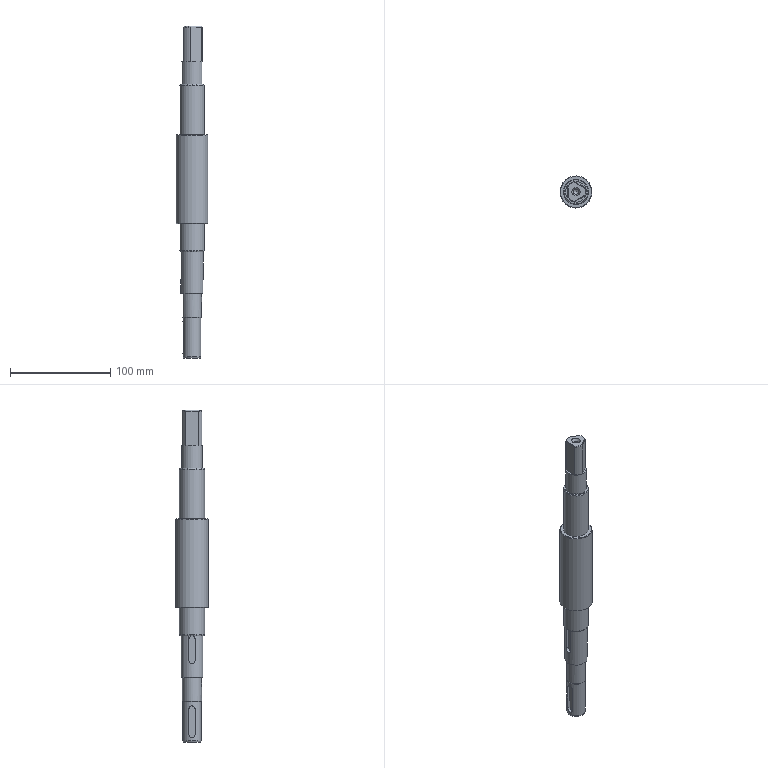NC program | NX | posted with a generic post | part box 32 x 32 x 331.3 mm
Whole program:
N10 G17 G21 G94 G90
(刀补6_COPY_1 , TOOL : D4)
N12 T04 M6
N14 G54
N16 G17 G0 G90 X89.748 Y0.433 B0. C0. S6685 M3
N18 G43 Z30. H4
N20 Z-3.547
N22 G94 G1 X89.648 Z-3.552 F1000.
N24 X89.554 Y0.431 Z-3.557
N26 X89.379 Y0.349 Z-3.567
N28 X89.318 Y0.277 Z-3.572
N30 X89.218 Y0. Z-3.587
N32 X89.318 Y-0.277 Z-3.603
N34 X89.378 Y-0.349 Z-3.608
N36 X89.49 Y-0.412 Z-3.614
N38 X89.594 Y-0.428 Z-3.62
N40 X89.652 Y-0.433 Z-3.623
N42 X101.588 Z-4.249
N44 X101.612 Y-0.413 Z-4.25
N46 X101.646 Y-0.411 Z-4.252
N48 X101.882 Y-0.359 Z-4.265
N50 X101.97 Y-0.307 Z-4.27
N52 X102.036 Y-0.209 Z-4.276
N54 X102.069 Y-0.119 Z-4.281
N56 X102.082 Y-0.002 Z-4.287
N58 X102.004 Y0.26 Z-4.302
N60 X101.952 Y0.326 Z-4.306
N62 X101.883 Y0.364 Z-4.31
N64 X101.828 Y0.393 Z-4.313
N66 X101.701 Y0.433 Z-4.32
N68 X95.875 Z-4.626
N70 G41 X95.776 Y0.45 D4
N72 X89.648 F1650.
N74 G3 X89.303 Y0.285 R0.457
N76 G1 X89.2 Y0.
N78 X89.303 Y-0.285
N80 G3 X89.592 Y-0.446 R0.454
N82 G1 X89.648 Y-0.45
N84 X101.594
N86 X101.615 Y-0.425
N88 X101.647 Y-0.43
N90 X101.649 Y-0.428
N92 X101.888 Y-0.375
N94 X101.982 Y-0.32
N96 G3 X102.1 Y0. R0.712
N98 G1 X102.043 Y0.19
N100 G3 X101.892 Y0.38 R0.324
N102 G1 X101.835 Y0.409
N104 X101.703 Y0.45
N106 X95.776
N108 X91.247 Z-4.705
N110 X89.648
N112 G3 X89.303 Y0.285 R0.457
N114 G1 X89.2 Y0.
N116 X89.303 Y-0.285
N118 G3 X89.592 Y-0.446 R0.454
N120 G1 X89.648 Y-0.45
N122 X101.594
N124 X101.612 Y-0.437
N126 X101.888 Y-0.375
N128 X101.986 Y-0.314
N130 G3 X102.1 Y0. R0.709
N132 G1 X102.043 Y0.19
N134 G3 X101.892 Y0.38 R0.324
N136 G1 X101.835 Y0.409
N138 X101.703 Y0.45
N140 X95.776
N142 X91.247 Z-4.784
N144 X89.648
N146 G3 X89.303 Y0.285 R0.457
N148 G1 X89.2 Y0.
N150 X89.303 Y-0.285
N152 G3 X89.592 Y-0.446 R0.454
N154 G1 X89.648 Y-0.45
N156 X101.594
N158 X101.612 Y-0.437
N160 X101.888 Y-0.375
N162 X101.986 Y-0.314
N164 G3 X102.1 Y0. R0.709
N166 G1 X102.043 Y0.19
N168 G3 X101.892 Y0.38 R0.324
N170 G1 X101.835 Y0.409
N172 X101.703 Y0.45
N174 X95.776
N176 X91.247 Z-4.863
N178 X89.648
N180 G3 X89.303 Y0.285 R0.457
N182 G1 X89.2 Y0.
N184 X89.303 Y-0.285
N186 G3 X89.592 Y-0.446 R0.454
N188 G1 X89.648 Y-0.45
N190 X101.594
N192 X101.612 Y-0.437
N194 X101.888 Y-0.375
N196 X101.986 Y-0.314
N198 G3 X102.1 Y0. R0.709
N200 G1 X102.043 Y0.19
N202 G3 X101.892 Y0.38 R0.324
N204 G1 X101.835 Y0.409
N206 X101.703 Y0.45
N208 X95.776
N210 X91.247 Z-4.942
N212 X89.648
N214 G3 X89.303 Y0.285 R0.457
N216 G1 X89.2 Y0.
N218 X89.303 Y-0.285
N220 G3 X89.592 Y-0.446 R0.454
N222 G1 X89.648 Y-0.45
N224 X101.594
N226 X101.612 Y-0.437
N228 X101.888 Y-0.375
N230 X101.986 Y-0.314
N232 G3 X102.1 Y0. R0.709
N234 G1 X102.043 Y0.19
N236 G3 X101.892 Y0.38 R0.324
N238 G1 X101.835 Y0.409
N240 X101.703 Y0.45
N242 X95.776
N244 X91.247 Z-5.021
N246 X89.65
N248 G3 X89.2 Y0. R0.45
N250 X89.65 Y-0.45 R0.45
N252 G1 X101.594
N254 X101.612 Y-0.437
N256 X101.888 Y-0.375
N258 X101.985 Y-0.315
N260 G3 X102.1 Y0. R0.71
N262 G1 X102.043 Y0.19
N264 G3 X101.892 Y0.38 R0.324
N266 G1 X101.835 Y0.409
N268 X101.703 Y0.45
N270 X95.776
N272 X91.247 Z-5.1
N274 X89.65
N276 G3 X89.2 Y0. R0.45
N278 X89.65 Y-0.45 R0.45
N280 G1 X101.594
N282 X101.612 Y-0.437
N284 X101.888 Y-0.375
N286 X101.985 Y-0.316
N288 G3 X102.1 Y0. R0.71
N290 G1 X102.041 Y0.197
N292 G3 X101.9 Y0.374 R0.303
N294 G1 X101.835 Y0.409
N296 X101.703 Y0.45
N298 X95.776
N300 X91.247 Z-5.179
N302 X89.65
N304 G3 X89.2 Y0. R0.45
N306 X89.65 Y-0.45 R0.45
N308 G1 X101.594
N310 X101.612 Y-0.437
N312 X101.888 Y-0.375
N314 X101.984 Y-0.317
N316 G3 X102.1 Y0. R0.71
N318 G1 X102.042 Y0.195
N320 G3 X101.919 Y0.361 R0.303
N322 G1 X101.884 Y0.383
N324 X101.835 Y0.409
N326 X101.703 Y0.45
N328 X95.776
N330 X91.247 Z-5.258
N332 X89.65
N334 G3 X89.2 Y0. R0.45
N336 X89.65 Y-0.45 R0.45
N338 G1 X101.594
N340 X101.612 Y-0.437
N342 X101.888 Y-0.375
N344 X101.984 Y-0.317
N346 G3 X102.1 Y0. R0.711
N348 G1 X102.042 Y0.195
N350 G3 X101.919 Y0.361 R0.303
N352 G1 X101.88 Y0.386
N354 X101.835 Y0.409
N356 X101.703 Y0.45
N358 X95.776
N360 X91.247 Z-5.337
N362 X89.65
N364 G3 X89.2 Y0. R0.45
N366 X89.65 Y-0.45 R0.45
N368 G1 X101.594
N370 X101.612 Y-0.437
N372 X101.888 Y-0.375
N374 X101.984 Y-0.318
N376 G3 X102.1 Y0. R0.711
N378 G1 X102.042 Y0.195
N380 G3 X101.919 Y0.361 R0.303
N382 G1 X101.871 Y0.391
N384 X101.835 Y0.409
N386 X101.703 Y0.45
N388 X95.776
N390 X91.247 Z-5.416
N392 X89.65
N394 G3 X89.2 Y0. R0.45
N396 X89.65 Y-0.45 R0.45
N398 G1 X101.594
N400 X101.612 Y-0.437
N402 X101.888 Y-0.375
N404 X101.983 Y-0.319
N406 G3 X102.1 Y0. R0.712
N408 G1 X102.042 Y0.195
N410 G3 X101.919 Y0.361 R0.303
N412 G1 X101.871 Y0.391
N414 X101.835 Y0.409
N416 X101.703 Y0.45
N418 X95.776
N420 X91.247 Z-5.495
N422 X89.65
N424 G3 X89.2 Y0. R0.45
N426 X89.65 Y-0.45 R0.45
N428 G1 X101.594
N430 X101.612 Y-0.437
N432 X101.888 Y-0.375
N434 X101.983 Y-0.319
N436 G3 X102.1 Y0. R0.712
N438 G1 X102.042 Y0.195
N440 G3 X101.919 Y0.361 R0.303
N442 G1 X101.871 Y0.391
N444 X101.835 Y0.409
N446 X101.703 Y0.45
N448 X95.776
N450 X91.247 Z-5.575
N452 X89.65
N454 G3 X89.2 Y0. R0.45
N456 X89.65 Y-0.45 R0.45
N458 G1 X101.594
N460 X101.612 Y-0.437
N462 X101.888 Y-0.375
N464 X101.982 Y-0.32
N466 G3 X102.1 Y0. R0.712
N468 G1 X102.042 Y0.195
N470 G3 X101.919 Y0.361 R0.303
N472 G1 X101.892 Y0.38
N474 X101.835 Y0.409
N476 X101.703 Y0.45
N478 X95.776
N480 X91.247 Z-5.654
N482 X89.65
N484 G3 X89.2 Y0. R0.45
N486 X89.65 Y-0.45 R0.45
N488 G1 X101.594
N490 X101.612 Y-0.437
N492 X101.888 Y-0.374
N494 X101.982 Y-0.321
N496 G3 X102.1 Y0. R0.713
N498 G1 X102.042 Y0.195
N500 G3 X101.919 Y0.361 R0.303
N502 G1 X101.892 Y0.38
N504 X101.845 Y0.418
N506 X101.789 Y0.44
N508 X101.729 Y0.442
N510 X101.651 Y0.45
N512 X95.776
N514 X91.247 Z-5.733
N516 X89.65
N518 G3 X89.2 Y0. R0.45
N520 X89.65 Y-0.45 R0.45
N522 G1 X101.594
N524 X101.612 Y-0.437
N526 X101.888 Y-0.374
N528 X101.982 Y-0.321
N530 G3 X102.1 Y0. R0.713
N532 G1 X102.042 Y0.195
N534 G3 X101.919 Y0.361 R0.303
N536 G1 X101.892 Y0.38
N538 X101.845 Y0.418
N540 X101.789 Y0.44
N542 X101.729 Y0.442
N544 X101.651 Y0.45
N546 X95.776
N548 X91.247 Z-5.812
N550 X89.65
N552 G3 X89.2 Y0. R0.45
N554 X89.65 Y-0.45 R0.45
N556 G1 X101.594
N558 X101.612 Y-0.437
N560 X101.888 Y-0.374
N562 X101.981 Y-0.322
N564 G3 X102.1 Y0. R0.713
N566 G1 X102.042 Y0.195
N568 G3 X101.919 Y0.361 R0.303
N570 G1 X101.892 Y0.38
N572 X101.845 Y0.418
N574 X101.789 Y0.44
N576 X101.729 Y0.442
N578 X101.651 Y0.45
N580 X95.776
N582 X91.247 Z-5.891
N584 X89.65
N586 G3 X89.2 Y0. R0.45
N588 X89.65 Y-0.45 R0.45
N590 G1 X101.594
N592 X101.612 Y-0.437
N594 X101.888 Y-0.374
N596 X101.981 Y-0.323
N598 G3 X102.1 Y0. R0.714
N600 G1 X102.042 Y0.195
N602 G3 X101.919 Y0.361 R0.303
N604 G1 X101.892 Y0.38
N606 X101.845 Y0.418
N608 X101.789 Y0.44
N610 X101.729 Y0.442
N612 X101.651 Y0.45
N614 X95.776
N616 X91.247 Z-5.97
N618 X89.65
N620 G3 X89.2 Y0. R0.45
N622 X89.65 Y-0.45 R0.45
N624 G1 X101.594
N626 X101.612 Y-0.437
N628 X101.888 Y-0.374
N630 X101.98 Y-0.323
N632 G3 X102.1 Y0. R0.714
N634 G1 X102.042 Y0.195
N636 G3 X101.919 Y0.361 R0.303
N638 G1 X101.892 Y0.38
N640 X101.845 Y0.418
N642 X101.789 Y0.44
N644 X101.729 Y0.442
N646 X101.651 Y0.45
N648 X95.776
N650 X91.247 Z-6.049
N652 X89.65
N654 G3 X89.2 Y0. R0.45
N656 X89.65 Y-0.45 R0.45
N658 G1 X101.594
N660 X101.612 Y-0.437
N662 X101.888 Y-0.374
N664 X101.98 Y-0.324
N666 G3 X102.1 Y0. R0.715
N668 G1 X102.042 Y0.195
N670 G3 X101.919 Y0.361 R0.303
N672 G1 X101.892 Y0.38
N674 X101.845 Y0.418
N676 X101.789 Y0.44
N678 X101.729 Y0.442
N680 X101.651 Y0.45
N682 X95.776
N684 X91.247 Z-6.128
N686 X89.65
N688 G3 X89.2 Y0. R0.45
N690 X89.65 Y-0.45 R0.45
N692 G1 X101.594
N694 X101.612 Y-0.437
N696 X101.888 Y-0.374
N698 X101.98 Y-0.324
N700 G3 X102.1 Y0. R0.715
N702 G1 X102.042 Y0.195
N704 G3 X101.919 Y0.361 R0.303
N706 G1 X101.892 Y0.38
N708 X101.845 Y0.418
N710 X101.789 Y0.44
N712 X101.729 Y0.442
N714 X101.651 Y0.45
N716 X95.776
N718 X91.247 Z-6.207
N720 X89.65
N722 G3 X89.2 Y0. R0.45
N724 X89.65 Y-0.45 R0.45
N726 G1 X101.594
N728 X101.612 Y-0.437
N730 X101.888 Y-0.374
N732 X101.979 Y-0.325
N734 G3 X102.1 Y0. R0.715
N736 G1 X102.042 Y0.195
N738 G3 X101.919 Y0.361 R0.303
N740 G1 X101.892 Y0.38
N742 X101.845 Y0.418
N744 X101.789 Y0.44
N746 X101.729 Y0.442
N748 X101.651 Y0.45
N750 X95.776
N752 X91.247 Z-6.286
N754 X89.65
N756 G3 X89.2 Y0. R0.45
N758 X89.65 Y-0.45 R0.45
N760 G1 X101.632
N762 X101.648 Y-0.428
N764 X101.888 Y-0.374
N766 X101.979 Y-0.326
N768 G3 X102.1 Y0. R0.716
N770 G1 X102.042 Y0.195
N772 G3 X101.919 Y0.361 R0.303
N774 G1 X101.892 Y0.38
N776 X101.845 Y0.418
N778 X101.789 Y0.44
N780 X101.729 Y0.442
N782 X101.651 Y0.45
N784 X95.776
N786 X91.247 Z-6.365
N788 X89.65
N790 G3 X89.2 Y0. R0.45
N792 X89.65 Y-0.45 R0.45
N794 G1 X101.63
N796 X101.648 Y-0.428
N798 X101.888 Y-0.374
N800 X101.979 Y-0.326
N802 G3 X102.1 Y0. R0.716
N804 G1 X102.042 Y0.195
N806 G3 X101.919 Y0.361 R0.303
N808 G1 X101.892 Y0.38
N810 G3 X101.65 Y0.45 R0.435
N812 G1 X95.776
N814 X91.247 Z-6.444
N816 X89.65
N818 G3 X89.2 Y0. R0.45
N820 X89.65 Y-0.45 R0.45
N822 G1 X101.63
N824 X101.648 Y-0.428
N826 X101.888 Y-0.374
N828 X101.897 Y-0.369
N830 X101.955 Y-0.344
N832 X102. Y-0.3
N834 X102.028 Y-0.243
N836 X102.1 Y0.
N838 X102.042 Y0.195
N840 G3 X101.919 Y0.361 R0.303
N842 G1 X101.892 Y0.38
N844 G3 X101.65 Y0.45 R0.435
N846 G1 X95.776
N848 X91.247 Z-6.523
N850 X89.65
N852 G3 X89.2 Y0. R0.45
N854 X89.65 Y-0.45 R0.45
N856 G1 X101.63
N858 X101.648 Y-0.428
N860 X101.888 Y-0.374
N862 X101.9
N864 G3 X101.65 Y0.45 R0.45
N866 G1 X95.776
N868 X91.247 Z-6.602
N870 X89.65
N872 G3 X89.2 Y0. R0.45
N874 X89.65 Y-0.45 R0.45
N876 G1 X101.63
N878 X101.648 Y-0.428
N880 X101.888 Y-0.374
N882 X101.9
N884 G3 X101.65 Y0.45 R0.45
N886 G1 X95.776
N888 X91.247 Z-6.681
N890 X89.65
N892 G3 X89.2 Y0. R0.45
N894 X89.65 Y-0.45 R0.45
N896 G1 X101.63
N898 X101.648 Y-0.428
N900 X101.888 Y-0.374
N902 X101.9
N904 G3 X101.65 Y0.45 R0.45
N906 G1 X95.776
N908 X91.247 Z-6.761
N910 X89.65
N912 G3 X89.2 Y0. R0.45
N914 X89.65 Y-0.45 R0.45
N916 G1 X101.63
N918 X101.648 Y-0.428
N920 X101.888 Y-0.374
N922 X101.9
N924 G3 X101.65 Y0.45 R0.45
N926 G1 X95.776
N928 X91.247 Z-6.84
N930 X89.65
N932 G3 X89.2 Y0. R0.45
N934 X89.65 Y-0.45 R0.45
N936 G1 X101.63
N938 X101.648 Y-0.428
N940 X101.888 Y-0.374
N942 X101.9
N944 G3 X101.65 Y0.45 R0.45
N946 G1 X95.776
N948 X91.247 Z-6.919
N950 X89.65
N952 G3 X89.2 Y0. R0.45
N954 X89.65 Y-0.45 R0.45
N956 G1 X101.63
N958 X101.648 Y-0.428
N960 X101.888 Y-0.374
N962 X101.9
N964 G3 X101.65 Y0.45 R0.45
N966 G1 X95.776
N968 X91.247 Z-6.998
N970 X89.65
N972 G3 X89.2 Y0. R0.45
N974 X89.65 Y-0.45 R0.45
N976 G1 X101.63
N978 X101.648 Y-0.428
N980 X101.888 Y-0.374
N982 X101.9
N984 G3 X101.65 Y0.45 R0.45
N986 G1 X95.776
N988 X91.247 Z-7.077
N990 X89.65
N992 G3 X89.2 Y0. R0.45
N994 X89.65 Y-0.45 R0.45
N996 G1 X101.63
N998 X101.648 Y-0.428
N1000 X101.888 Y-0.374
N1002 X101.9
N1004 G3 X101.65 Y0.45 R0.45
N1006 G1 X95.776
N1008 X91.247 Z-7.156
N1010 X89.65
N1012 G3 X89.2 Y0. R0.45
N1014 X89.65 Y-0.45 R0.45
N1016 G1 X101.63
N1018 X101.648 Y-0.428
N1020 X101.888 Y-0.374
N1022 X101.9
N1024 G3 X101.65 Y0.45 R0.45
N1026 G1 X95.776
N1028 X91.247 Z-7.235
N1030 X89.65
N1032 G3 X89.2 Y0. R0.45
N1034 X89.65 Y-0.45 R0.45
N1036 G1 X101.63
N1038 X101.647 Y-0.429
N1040 X101.888 Y-0.374
N1042 X101.9
N1044 G3 X101.65 Y0.45 R0.45
N1046 G1 X95.776
N1048 X91.247 Z-7.314
N1050 X89.65
N1052 G3 X89.2 Y0. R0.45
N1054 X89.65 Y-0.45 R0.45
N1056 G1 X101.63
N1058 X101.647 Y-0.429
N1060 X101.888 Y-0.374
N1062 X101.9
N1064 G3 X101.65 Y0.45 R0.45
N1066 G1 X95.776
N1068 X91.247 Z-7.393
N1070 X89.65
N1072 G3 X89.2 Y0. R0.45
N1074 X89.65 Y-0.45 R0.45
N1076 G1 X101.63
N1078 X101.647 Y-0.429
N1080 X101.888 Y-0.374
N1082 X101.9
N1084 G3 X101.65 Y0.45 R0.45
N1086 G1 X95.776
N1088 X91.247 Z-7.472
N1090 X89.65
N1092 G3 X89.2 Y0. R0.45
N1094 X89.65 Y-0.45 R0.45
N1096 G1 X101.63
N1098 X101.647 Y-0.429
N1100 X101.888 Y-0.374
N1102 X101.9
N1104 G3 X101.65 Y0.45 R0.45
N1106 G1 X95.776
N1108 X91.247 Z-7.551
N1110 X89.65
N1112 G3 X89.2 Y0. R0.45
N1114 X89.65 Y-0.45 R0.45
N1116 G1 X101.63
N1118 X101.647 Y-0.429
N1120 X101.888 Y-0.374
N1122 X101.9
N1124 G3 X101.65 Y0.45 R0.45
N1126 G1 X95.776
N1128 X91.247 Z-7.63
N1130 X89.65
N1132 G3 X89.2 Y0. R0.45
N1134 X89.65 Y-0.45 R0.45
N1136 G1 X101.63
N1138 X101.647 Y-0.429
N1140 X101.888 Y-0.373
N1142 X101.9 Y-0.374
N1144 G3 X101.65 Y0.45 R0.45
N1146 G1 X95.776
N1148 X91.247 Z-7.709
N1150 X89.65
N1152 G3 X89.2 Y0. R0.45
N1154 X89.65 Y-0.45 R0.45
N1156 G1 X101.63
N1158 X101.647 Y-0.429
N1160 X101.888 Y-0.373
N1162 X101.9 Y-0.374
N1164 G3 X101.65 Y0.45 R0.45
N1166 G1 X95.776
N1168 X91.247 Z-7.788
N1170 X89.65
N1172 G3 X89.2 Y0. R0.45
N1174 X89.65 Y-0.45 R0.45
N1176 G1 X101.63
N1178 X101.647 Y-0.429
N1180 X101.888 Y-0.373
N1182 X101.9 Y-0.374
N1184 G3 X101.65 Y0.45 R0.45
N1186 G1 X95.776
N1188 X91.247 Z-7.867
N1190 X89.65
N1192 G3 X89.2 Y0. R0.45
N1194 X89.65 Y-0.45 R0.45
N1196 G1 X101.63
N1198 X101.647 Y-0.428
N1200 X101.888 Y-0.373
N1202 X101.9 Y-0.374
N1204 G3 X101.65 Y0.45 R0.45
N1206 G1 X95.776
N1208 X91.247 Z-7.947
N1210 X89.65
N1212 G3 X89.2 Y0. R0.45
N1214 X89.65 Y-0.45 R0.45
N1216 G1 X101.63
N1218 X101.647 Y-0.428
N1220 X101.888 Y-0.373
N1222 X101.9 Y-0.374
N1224 G3 X101.65 Y0.45 R0.45
N1226 G1 X95.776
N1228 X91.247 Z-8.026
N1230 X89.65
N1232 G3 X89.2 Y0. R0.45
N1234 X89.65 Y-0.45 R0.45
N1236 G1 X101.63
N1238 X101.647 Y-0.428
N1240 X101.888 Y-0.373
N1242 X101.9 Y-0.374
N1244 G3 X101.65 Y0.45 R0.45
N1246 G1 X95.776
N1248 X91.247 Z-8.105
N1250 X89.65
N1252 G3 X89.2 Y0. R0.45
N1254 X89.65 Y-0.45 R0.45
N1256 G1 X101.63
N1258 X101.647 Y-0.428
N1260 X101.888 Y-0.373
N1262 X101.9 Y-0.374
N1264 G3 X101.65 Y0.45 R0.45
N1266 G1 X95.776
N1268 X91.247 Z-8.184
N1270 X89.65
N1272 G3 X89.2 Y0. R0.45
N1274 X89.65 Y-0.45 R0.45
N1276 G1 X101.63
N1278 X101.647 Y-0.428
N1280 X101.888 Y-0.373
N1282 X101.9 Y-0.374
N1284 G3 X101.65 Y0.45 R0.45
N1286 G1 X95.776
N1288 X91.247 Z-8.263
N1290 X89.65
N1292 G3 X89.2 Y0. R0.45
N1294 X89.65 Y-0.45 R0.45
N1296 G1 X101.63
N1298 X101.647 Y-0.428
N1300 X101.888 Y-0.373
N1302 X101.9 Y-0.374
N1304 G3 X101.65 Y0.45 R0.45
N1306 G1 X95.776
N1308 X91.247 Z-8.342
N1310 X89.65
N1312 G3 X89.2 Y0. R0.45
N1314 X89.65 Y-0.45 R0.45
N1316 G1 X101.63
N1318 X101.647 Y-0.428
N1320 X101.888 Y-0.373
N1322 X101.9 Y-0.374
N1324 G3 X101.65 Y0.45 R0.45
N1326 G1 X95.776
N1328 X91.247 Z-8.421
N1330 X89.65
N1332 G3 X89.2 Y0. R0.45
N1334 X89.65 Y-0.45 R0.45
N1336 G1 X101.63
N1338 X101.647 Y-0.428
N1340 X101.888 Y-0.373
N1342 X101.9 Y-0.374
N1344 G3 X101.65 Y0.45 R0.45
N1346 G1 X95.776
N1348 X91.247 Z-8.5
N1350 X89.65
N1352 G3 X89.2 Y0. R0.45
N1354 X89.65 Y-0.45 R0.45
N1356 G1 X101.63
N1358 X101.647 Y-0.428
N1360 X101.888 Y-0.373
N1362 X101.9 Y-0.374
N1364 G3 X101.65 Y0.45 R0.45
N1366 G1 X91.247
N1368 G40
N1370 X91.148 Y0.433
N1372 Z-7.5
N1374 G0 Z30.
N1376 M5
N1378 M2